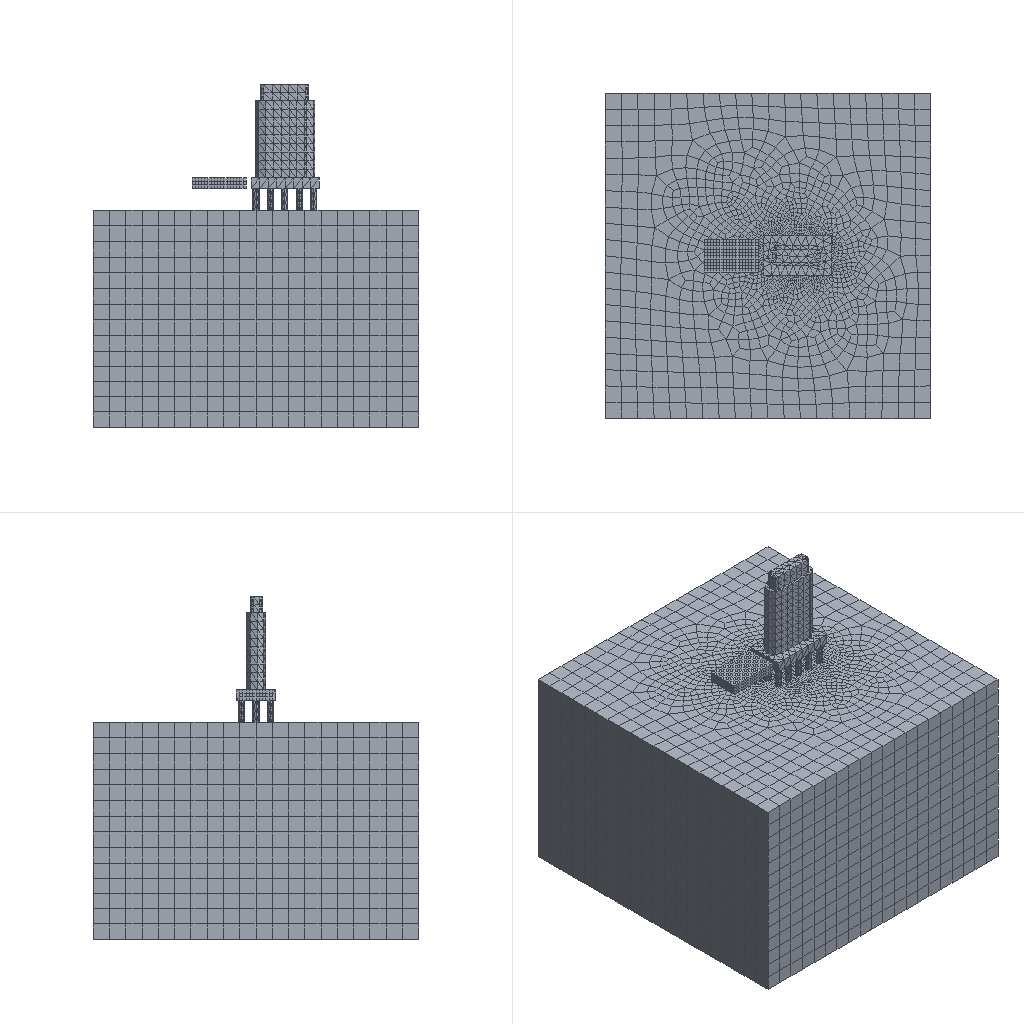Simulation study | abaqus
Set-up summary:
category,name,step,type,value,unit,region
solver,abaqus
solver,version,,,Abaqus/Explicit 2020
units,not stated in the deck,,not stated
analysis,deck,,transient,transient
load_step,Step-1,Step-1,transient,nlgeom=True
contact,interactions,,,general=1 pairs=0 ties=0
load_step,requested,,,1
mesh,nodes,,,35219
mesh,elements,,,40983
element_type,C3D4,,solid,13041
element_type,C3D8R,,solid,27942
load,load commands in deck,,count,1
bc,support commands in deck,,count,3
material,BING,,in results
material,SOIL,,in results
material,ZHUANG,,in results
check,setup vs results,,match,"per instance, exact: element labels, types and connectivity; labels of the nodes the elements use; coordinates of those nodes at SINGLE_PRECISION in 3 of 3 instance(s)"
Abaqus input file, long lists of numbers shortened:
*Heading
** Job name: Job-1 Model name: Model-1
** Generated by: Abaqus/CAE 2020
*Preprint, echo=NO, model=NO, history=NO, contact=NO
**
** PARTS
**
*Part, name=work-1
*Node
      1,   266.8,   52.7,        -650.
      2,   252.8,   66.7,        -650.
** (30448 more lines like these left out)
*Element, type=C3D8R
    1,  1574,  1595,  1479,    37,  8948,  8969,  8853,   547
    2,   187,    37,  1479,  1634,  5041,   547,  8853,  9008
** (27430 more lines like these left out)
*Nset, nset=Set-1, generate
     1,  30450,      1
*Elset, elset=Set-1, generate
     1,  27432,      1
** Section: soil
*Solid Section, elset=Set-1, material=soil
,
*End Part
**
*Part, name=work-22
*Node
      1,        -325.,         -75.,         150.
      2,  -310.294,         -75.,         150.
** (790 more lines like these left out)
*Element, type=C3D8R
  1, 199, 200, 218, 217,   1,   2,  20,  19
  2, 200, 201, 219, 218,   2,   3,  21,  20
** (508 more lines like these left out)
*Nset, nset=Set-1, generate
   1,  792,    1
*Elset, elset=Set-1, generate
   1,  510,    1
** Section: bing
*Solid Section, elset=Set-1, material=bing
,
*End Part
**
*Part, name=zhuangji
*Node
      1,   19.2,   9.48,   578.45
      2,   19.2,  -15.48,   578.45
** (3975 more lines like these left out)
*Element, type=C3D4
    1, 3229, 3230, 3231, 3232
    2, 3229, 3233, 1380, 3234
** (13039 more lines like these left out)
*Nset, nset=Set-4, generate
    1,  3977,     1
*Elset, elset=Set-4, generate
     1,  13041,      1
** Section: zhuang
*Solid Section, elset=Set-4, material=zhuang
,
*End Part
**
**
** ASSEMBLY
**
*Assembly, name=Assembly
**
*Instance, name=work-1-1, part=work-1
*End Instance
**
*Instance, name=work-22-1, part=work-22
         30.,           0.,           0.
*End Instance
**
*Instance, name=zhuangji-1, part=zhuangji
*End Instance
**
*Nset, nset=Set-1, instance=work-1-1
  129,  130,  131,  132,  133,  134,  135,  136,  137,  138,  139,  140,  141,  142,  143,  144
  145,  146,  147,  932,  933,  934,  935,  936,  937,  938,  943,  944,  945,  946,  947,  948
** (126 more lines like these left out)
*Elset, elset=Set-1, instance=work-1-1
 17459, 17460, 17461, 17462, 25215, 25216, 25217, 25218, 25219, 25220, 25221, 25222, 25223, 25224, 25225, 25226
 25227, 25228, 25229, 25230, 25231, 25232, 25233, 25234, 25235, 25236, 25237, 25238, 25239, 25240, 25241, 25242
** (123 more lines like these left out)
*Nset, nset=Set-2, instance=work-1-1
   61,   62,   63,   64,   65,   66,   67,   68,  130,  131,  146,  147,  208,  209,  210,  211
  212,  213,  214,  215,  216,  217,  218,  219,  220,  221,  222,  223,  224,  225,  226,  246
** (38 more lines like these left out)
*Elset, elset=Set-2, instance=work-1-1
    28,    29,    30,   113,   114,   220,   221,   222,   256,   278,   279,   280,   299,   304,   305,   319
   320,   328,   329,   340,   345,   349,   350,   374,   381,   382,   390,   391,   392,   398,   403,   407
** (33 more lines like these left out)
*Nset, nset=Set-3, instance=work-1-1
   61,   62,   63,   64,   65,   66,   67,   68,  130,  131,  146,  147,  227,  228,  229,  230
  231,  232,  233,  234,  235,  236,  237,  238,  239,  240,  241,  242,  243,  244,  245,  265
** (38 more lines like these left out)
*Elset, elset=Set-3, instance=work-1-1
    36,    37,    38,    73,    74,    75,   112,   113,   150,   151,   152,   169,   170,   256,   270,   271
   285,   286,   344,   345,   346,   351,   353,   354,   359,   363,   368,   372,   373,   397,   402,   403
** (33 more lines like these left out)
*Nset, nset=Set-4, instance=work-22-1, generate
   1,  792,    1
*Elset, elset=Set-4, instance=work-22-1, generate
   1,  510,    1
*End Assembly
**
** MATERIALS
**
*Material, name=bing
*Brittle Cracking
  1.,    0.
 1.5, 5e-05
*Brittle Shear
  1.,    0.
 0.8, 4e-05
*Brittle Failure
 1e-07,
*Density
 9e-10,
*Elastic
5000., 0.33
*Material, name=soil
*Density
 1.9e-09,
*Elastic
2000., 0.36
*Material, name=zhuang
*Density
 2.6e-09,
*Elastic
20000., 0.33
**
** INTERACTION PROPERTIES
**
*Surface Interaction, name=IntProp-1
*Friction
 0.1,
*Surface Behavior, pressure-overclosure=HARD
**
** PREDEFINED FIELDS
**
** Name: Predefined Field-1   Type: Velocity
*Initial Conditions, type=VELOCITY
Set-4, 1, 250.
** ----------------------------------------------------------------
**
** STEP: Step-1
**
*Step, name=Step-1, nlgeom=YES
*Dynamic, Explicit
, 0.11
*Bulk Viscosity
0.06, 1.2
** Mass Scaling: Semi-Automatic
**               Whole Model
*Fixed Mass Scaling, factor=50.
**
** BOUNDARY CONDITIONS
**
** Name: BC-1 Type: 位移/转角
*Boundary
Set-1, 3, 3
** Name: BC-2 Type: 位移/转角
*Boundary
Set-2, 1, 1
** Name: BC-3 Type: 位移/转角
*Boundary
Set-3, 2, 2
**
** INTERACTIONS
**
** Interaction: Int-1
*Contact, op=NEW
*Contact Inclusions, ALL EXTERIOR
*Contact Property Assignment
 ,  , IntProp-1
**
** OUTPUT REQUESTS
**
*Restart, write, number interval=1, time marks=NO
**
** FIELD OUTPUT: F-Output-1
**
*Output, field, number interval=30
*Node Output
A, CF, RF, RM, RT, U, V
*Element Output, directions=YES
E, EDCDEN, EDT, ELEDEN, ELEN, ENER, EVF, LE, MISES, MISESMAX, MISESONLY, NE, PE, PEEQ, PEEQMAX, PEEQT
PEEQVAVG, PEMAG, PEQC, PEVAVG, PRESSONLY, S, SEQUT, SF, SFABRIC, SSAVG, STATUS, SVAVG, YIELDPOT
*Contact Output
CDISP, CFORCE, CSTRESS, CTHICK, FSLIP, FSLIPR, PPRESS
**
** HISTORY OUTPUT: H-Output-1
**
*Output, history, variable=PRESELECT
*End Step
Results summary:
result,step,Step-1,completed,increments=21283 time=0.11/0.11
result,analysis,,,transient
result,last_loadstep,,,1
result,analysis steps,,count,1
result,primary field,,,U
result,reaction total,,FX,-5246.49,model units
result,reaction total,,FY,219.001,model units
result,reaction total,,FZ,-310.354,model units